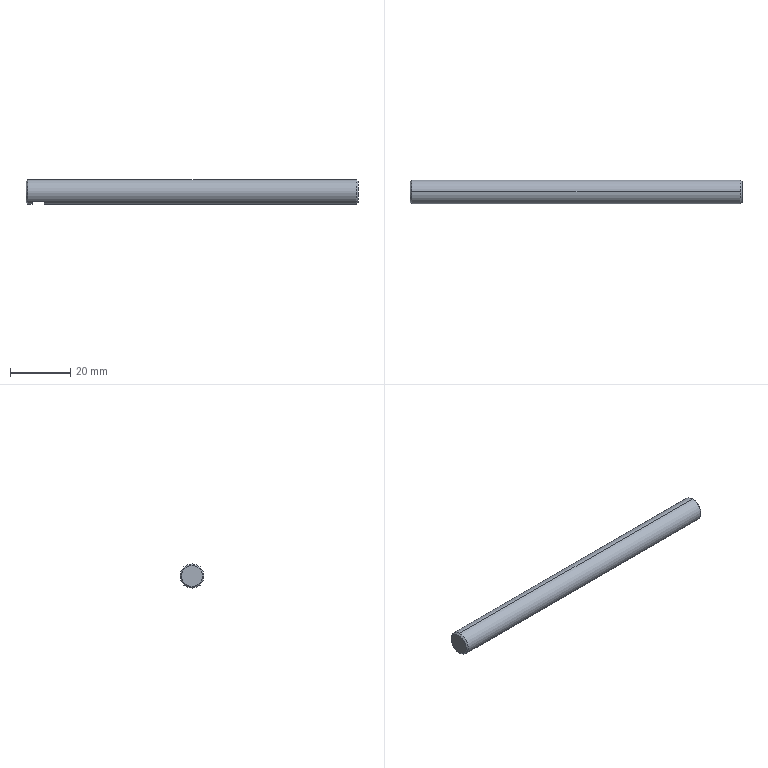Part | SolidWorks | features Chamfer 1, ICE 1, Revolution 1 | 1 solid | 11 faces | box 110 x 8 x 8 mm | volume 5509 mm3 | plane 5 | cone 4 | cylinder 2 | commonest cylinder face diameters 8 x2
STEP:
#1=CARTESIAN_POINT('',(0.,0.,3.5));
#2=VERTEX_POINT('',#1);
#3=CARTESIAN_POINT('',(0.,0.,-3.5));
#4=VERTEX_POINT('',#3);
#5=CARTESIAN_POINT('',(0.,0.,0.));
#6=DIRECTION('',(-1.,0.,0.));
#7=DIRECTION('',(0.,0.,-1.));
#8=AXIS2_PLACEMENT_3D('',#5,#6,#7);
#9=CIRCLE('',#8,3.5);
#10=EDGE_CURVE('',#2,#4,#9,.T.);
#11=ORIENTED_EDGE('',*,*,#10,.F.);
#12=CARTESIAN_POINT('',(0.5,0.,4.));
#13=VERTEX_POINT('',#12);
#14=CARTESIAN_POINT('',(0.,0.,3.5));
#15=DIRECTION('',(0.7071,0.,0.7071));
#16=VECTOR('',#15,1000.);
#17=LINE('',#14,#16);
#18=EDGE_CURVE('',#2,#13,#17,.T.);
#19=ORIENTED_EDGE('',*,*,#18,.T.);
#20=CARTESIAN_POINT('',(0.5,0.,-4.));
#21=VERTEX_POINT('',#20);
#22=CARTESIAN_POINT('',(0.5,0.,0.));
#23=DIRECTION('',(1.,0.,0.));
#24=DIRECTION('',(0.,0.,-1.));
#25=AXIS2_PLACEMENT_3D('',#22,#23,#24);
#26=CIRCLE('',#25,4.);
#27=EDGE_CURVE('',#21,#13,#26,.T.);
#28=ORIENTED_EDGE('',*,*,#27,.F.);
#29=CARTESIAN_POINT('',(0.,0.,-3.5));
#30=DIRECTION('',(0.7071,0.,-0.7071));
#31=VECTOR('',#30,1000.);
#32=LINE('',#29,#31);
#33=EDGE_CURVE('',#4,#21,#32,.T.);
#34=ORIENTED_EDGE('',*,*,#33,.F.);
#35=EDGE_LOOP('',(#11,#19,#28,#34));
#36=FACE_OUTER_BOUND('',#35,.T.);
#37=CARTESIAN_POINT('',(0.,0.,0.));
#38=DIRECTION('',(1.,0.,0.));
#39=DIRECTION('',(0.,0.,-1.));
#40=AXIS2_PLACEMENT_3D('',#37,#38,#39);
#41=CONICAL_SURFACE('',#40,3.5,0.7854);
#42=ADVANCED_FACE('',(#36),#41,.T.);
#43=CARTESIAN_POINT('',(110.,0.,-3.5));
#44=VERTEX_POINT('',#43);
#45=CARTESIAN_POINT('',(110.,0.,3.5));
#46=VERTEX_POINT('',#45);
#47=CARTESIAN_POINT('',(110.,0.,0.));
#48=DIRECTION('',(1.,0.,0.));
#49=DIRECTION('',(0.,0.,1.));
#50=AXIS2_PLACEMENT_3D('',#47,#48,#49);
#51=CIRCLE('',#50,3.5);
#52=EDGE_CURVE('',#44,#46,#51,.T.);
#53=ORIENTED_EDGE('',*,*,#52,.F.);
#54=CARTESIAN_POINT('',(109.5,0.,-4.));
#55=VERTEX_POINT('',#54);
#56=CARTESIAN_POINT('',(109.5,0.,-4.));
#57=DIRECTION('',(-0.7071,0.,-0.7071));
#58=VECTOR('',#57,1000.);
#59=LINE('',#56,#58);
#60=EDGE_CURVE('',#44,#55,#59,.T.);
#61=ORIENTED_EDGE('',*,*,#60,.T.);
#62=CARTESIAN_POINT('',(109.5,0.,4.));
#63=VERTEX_POINT('',#62);
#64=CARTESIAN_POINT('',(109.5,0.,0.));
#65=DIRECTION('',(-1.,0.,0.));
#66=DIRECTION('',(0.,0.,1.));
#67=AXIS2_PLACEMENT_3D('',#64,#65,#66);
#68=CIRCLE('',#67,4.);
#69=EDGE_CURVE('',#63,#55,#68,.T.);
#70=ORIENTED_EDGE('',*,*,#69,.F.);
#71=CARTESIAN_POINT('',(109.5,0.,4.));
#72=DIRECTION('',(-0.7071,0.,0.7071));
#73=VECTOR('',#72,1000.);
#74=LINE('',#71,#73);
#75=EDGE_CURVE('',#46,#63,#74,.T.);
#76=ORIENTED_EDGE('',*,*,#75,.F.);
#77=EDGE_LOOP('',(#53,#61,#70,#76));
#78=FACE_OUTER_BOUND('',#77,.T.);
#79=CARTESIAN_POINT('',(109.5,0.,0.));
#80=DIRECTION('',(-1.,0.,0.));
#81=DIRECTION('',(0.,0.,1.));
#82=AXIS2_PLACEMENT_3D('',#79,#80,#81);
#83=CONICAL_SURFACE('',#82,4.,0.7854);
#84=ADVANCED_FACE('',(#78),#83,.T.);
#85=ORIENTED_EDGE('',*,*,#69,.T.);
#86=CARTESIAN_POINT('',(6.,0.,-4.));
#87=VERTEX_POINT('',#86);
#88=CARTESIAN_POINT('',(0.,0.,-4.));
#89=DIRECTION('',(-1.,0.,0.));
#90=VECTOR('',#89,1000.);
#91=LINE('',#88,#90);
#92=EDGE_CURVE('',#55,#87,#91,.T.);
#93=ORIENTED_EDGE('',*,*,#92,.T.);
#94=CARTESIAN_POINT('',(6.,2.646,-3.));
#95=VERTEX_POINT('',#94);
#96=CARTESIAN_POINT('',(6.,0.,0.));
#97=DIRECTION('',(1.,0.,0.));
#98=DIRECTION('',(0.,0.,-1.));
#99=AXIS2_PLACEMENT_3D('',#96,#97,#98);
#100=CIRCLE('',#99,4.);
#101=EDGE_CURVE('',#87,#95,#100,.T.);
#102=ORIENTED_EDGE('',*,*,#101,.T.);
#103=CARTESIAN_POINT('',(2.,2.646,-3.));
#104=VERTEX_POINT('',#103);
#105=CARTESIAN_POINT('',(0.,2.646,-3.));
#106=DIRECTION('',(-1.,0.,0.));
#107=VECTOR('',#106,1000.);
#108=LINE('',#105,#107);
#109=EDGE_CURVE('',#95,#104,#108,.T.);
#110=ORIENTED_EDGE('',*,*,#109,.T.);
#111=CARTESIAN_POINT('',(2.,0.,-4.));
#112=VERTEX_POINT('',#111);
#113=CARTESIAN_POINT('',(2.,0.,0.));
#114=DIRECTION('',(-1.,0.,0.));
#115=DIRECTION('',(0.,0.,1.));
#116=AXIS2_PLACEMENT_3D('',#113,#114,#115);
#117=CIRCLE('',#116,4.);
#118=EDGE_CURVE('',#104,#112,#117,.T.);
#119=ORIENTED_EDGE('',*,*,#118,.T.);
#120=CARTESIAN_POINT('',(0.,0.,-4.));
#121=DIRECTION('',(-1.,0.,0.));
#122=VECTOR('',#121,1000.);
#123=LINE('',#120,#122);
#124=EDGE_CURVE('',#112,#21,#123,.T.);
#125=ORIENTED_EDGE('',*,*,#124,.T.);
#126=ORIENTED_EDGE('',*,*,#27,.T.);
#127=CARTESIAN_POINT('',(0.,0.,4.));
#128=DIRECTION('',(-1.,0.,0.));
#129=VECTOR('',#128,1000.);
#130=LINE('',#127,#129);
#131=EDGE_CURVE('',#63,#13,#130,.T.);
#132=ORIENTED_EDGE('',*,*,#131,.F.);
#133=EDGE_LOOP('',(#85,#93,#102,#110,#119,#125,#126,#132));
#134=FACE_OUTER_BOUND('',#133,.T.);
#135=CARTESIAN_POINT('',(0.,0.,0.));
#136=DIRECTION('',(-1.,0.,0.));
#137=DIRECTION('',(0.,0.,1.));
#138=AXIS2_PLACEMENT_3D('',#135,#136,#137);
#139=CYLINDRICAL_SURFACE('',#138,4.);
#140=ADVANCED_FACE('',(#134),#139,.T.);
#141=CARTESIAN_POINT('',(0.,0.,0.));
#142=DIRECTION('',(-1.,0.,0.));
#143=DIRECTION('',(0.,0.,-1.));
#144=AXIS2_PLACEMENT_3D('',#141,#142,#143);
#145=CIRCLE('',#144,3.5);
#146=EDGE_CURVE('',#4,#2,#145,.T.);
#147=ORIENTED_EDGE('',*,*,#146,.T.);
#148=ORIENTED_EDGE('',*,*,#10,.T.);
#149=EDGE_LOOP('',(#147,#148));
#150=FACE_OUTER_BOUND('',#149,.T.);
#151=CARTESIAN_POINT('',(0.,0.,0.));
#152=DIRECTION('',(1.,0.,0.));
#153=DIRECTION('',(0.,0.,-1.));
#154=AXIS2_PLACEMENT_3D('',#151,#152,#153);
#155=PLANE('',#154);
#156=ADVANCED_FACE('',(#150),#155,.F.);
#157=ORIENTED_EDGE('',*,*,#92,.F.);
#158=CARTESIAN_POINT('',(109.5,0.,0.));
#159=DIRECTION('',(-1.,0.,0.));
#160=DIRECTION('',(0.,0.,1.));
#161=AXIS2_PLACEMENT_3D('',#158,#159,#160);
#162=CIRCLE('',#161,4.);
#163=EDGE_CURVE('',#55,#63,#162,.T.);
#164=ORIENTED_EDGE('',*,*,#163,.T.);
#165=ORIENTED_EDGE('',*,*,#131,.T.);
#166=CARTESIAN_POINT('',(0.5,0.,0.));
#167=DIRECTION('',(1.,0.,0.));
#168=DIRECTION('',(0.,0.,-1.));
#169=AXIS2_PLACEMENT_3D('',#166,#167,#168);
#170=CIRCLE('',#169,4.);
#171=EDGE_CURVE('',#13,#21,#170,.T.);
#172=ORIENTED_EDGE('',*,*,#171,.T.);
#173=ORIENTED_EDGE('',*,*,#124,.F.);
#174=CARTESIAN_POINT('',(2.,-2.646,-3.));
#175=VERTEX_POINT('',#174);
#176=CARTESIAN_POINT('',(2.,0.,0.));
#177=DIRECTION('',(-1.,0.,0.));
#178=DIRECTION('',(0.,0.,1.));
#179=AXIS2_PLACEMENT_3D('',#176,#177,#178);
#180=CIRCLE('',#179,4.);
#181=EDGE_CURVE('',#112,#175,#180,.T.);
#182=ORIENTED_EDGE('',*,*,#181,.T.);
#183=CARTESIAN_POINT('',(6.,-2.646,-3.));
#184=VERTEX_POINT('',#183);
#185=CARTESIAN_POINT('',(0.,-2.646,-3.));
#186=DIRECTION('',(1.,0.,0.));
#187=VECTOR('',#186,1000.);
#188=LINE('',#185,#187);
#189=EDGE_CURVE('',#175,#184,#188,.T.);
#190=ORIENTED_EDGE('',*,*,#189,.T.);
#191=CARTESIAN_POINT('',(6.,0.,0.));
#192=DIRECTION('',(1.,0.,0.));
#193=DIRECTION('',(0.,0.,-1.));
#194=AXIS2_PLACEMENT_3D('',#191,#192,#193);
#195=CIRCLE('',#194,4.);
#196=EDGE_CURVE('',#184,#87,#195,.T.);
#197=ORIENTED_EDGE('',*,*,#196,.T.);
#198=EDGE_LOOP('',(#157,#164,#165,#172,#173,#182,#190,#197));
#199=FACE_OUTER_BOUND('',#198,.T.);
#200=CARTESIAN_POINT('',(0.,0.,0.));
#201=DIRECTION('',(-1.,0.,0.));
#202=DIRECTION('',(0.,0.,1.));
#203=AXIS2_PLACEMENT_3D('',#200,#201,#202);
#204=CYLINDRICAL_SURFACE('',#203,4.);
#205=ADVANCED_FACE('',(#199),#204,.T.);
#206=CARTESIAN_POINT('',(110.,0.,0.));
#207=DIRECTION('',(1.,0.,0.));
#208=DIRECTION('',(0.,0.,1.));
#209=AXIS2_PLACEMENT_3D('',#206,#207,#208);
#210=CIRCLE('',#209,3.5);
#211=EDGE_CURVE('',#46,#44,#210,.T.);
#212=ORIENTED_EDGE('',*,*,#211,.T.);
#213=ORIENTED_EDGE('',*,*,#52,.T.);
#214=EDGE_LOOP('',(#212,#213));
#215=FACE_OUTER_BOUND('',#214,.T.);
#216=CARTESIAN_POINT('',(110.,4.,0.));
#217=DIRECTION('',(-1.,0.,0.));
#218=DIRECTION('',(0.,0.,1.));
#219=AXIS2_PLACEMENT_3D('',#216,#217,#218);
#220=PLANE('',#219);
#221=ADVANCED_FACE('',(#215),#220,.F.);
#222=CARTESIAN_POINT('',(6.,-5.,-3.));
#223=DIRECTION('',(0.,1.,0.));
#224=VECTOR('',#223,1000.);
#225=LINE('',#222,#224);
#226=EDGE_CURVE('',#184,#95,#225,.T.);
#227=ORIENTED_EDGE('',*,*,#226,.T.);
#228=ORIENTED_EDGE('',*,*,#101,.F.);
#229=ORIENTED_EDGE('',*,*,#196,.F.);
#230=EDGE_LOOP('',(#227,#228,#229));
#231=FACE_OUTER_BOUND('',#230,.T.);
#232=CARTESIAN_POINT('',(6.,-5.,-3.));
#233=DIRECTION('',(1.,0.,0.));
#234=DIRECTION('',(0.,0.,-1.));
#235=AXIS2_PLACEMENT_3D('',#232,#233,#234);
#236=PLANE('',#235);
#237=ADVANCED_FACE('',(#231),#236,.F.);
#238=ORIENTED_EDGE('',*,*,#226,.F.);
#239=ORIENTED_EDGE('',*,*,#189,.F.);
#240=CARTESIAN_POINT('',(2.,-5.,-3.));
#241=DIRECTION('',(0.,1.,0.));
#242=VECTOR('',#241,1000.);
#243=LINE('',#240,#242);
#244=EDGE_CURVE('',#175,#104,#243,.T.);
#245=ORIENTED_EDGE('',*,*,#244,.T.);
#246=ORIENTED_EDGE('',*,*,#109,.F.);
#247=EDGE_LOOP('',(#238,#239,#245,#246));
#248=FACE_OUTER_BOUND('',#247,.T.);
#249=CARTESIAN_POINT('',(2.,-5.,-3.));
#250=DIRECTION('',(0.,0.,1.));
#251=DIRECTION('',(1.,0.,0.));
#252=AXIS2_PLACEMENT_3D('',#249,#250,#251);
#253=PLANE('',#252);
#254=ADVANCED_FACE('',(#248),#253,.F.);
#255=ORIENTED_EDGE('',*,*,#244,.F.);
#256=ORIENTED_EDGE('',*,*,#181,.F.);
#257=ORIENTED_EDGE('',*,*,#118,.F.);
#258=EDGE_LOOP('',(#255,#256,#257));
#259=FACE_OUTER_BOUND('',#258,.T.);
#260=CARTESIAN_POINT('',(2.,-5.,-3.));
#261=DIRECTION('',(-1.,0.,0.));
#262=DIRECTION('',(0.,0.,1.));
#263=AXIS2_PLACEMENT_3D('',#260,#261,#262);
#264=PLANE('',#263);
#265=ADVANCED_FACE('',(#259),#264,.F.);
#266=ORIENTED_EDGE('',*,*,#60,.F.);
#267=ORIENTED_EDGE('',*,*,#211,.F.);
#268=ORIENTED_EDGE('',*,*,#75,.T.);
#269=ORIENTED_EDGE('',*,*,#163,.F.);
#270=EDGE_LOOP('',(#266,#267,#268,#269));
#271=FACE_OUTER_BOUND('',#270,.T.);
#272=CARTESIAN_POINT('',(109.5,0.,0.));
#273=DIRECTION('',(-1.,0.,0.));
#274=DIRECTION('',(0.,0.,1.));
#275=AXIS2_PLACEMENT_3D('',#272,#273,#274);
#276=CONICAL_SURFACE('',#275,4.,0.7854);
#277=ADVANCED_FACE('',(#271),#276,.T.);
#278=ORIENTED_EDGE('',*,*,#18,.F.);
#279=ORIENTED_EDGE('',*,*,#146,.F.);
#280=ORIENTED_EDGE('',*,*,#33,.T.);
#281=ORIENTED_EDGE('',*,*,#171,.F.);
#282=EDGE_LOOP('',(#278,#279,#280,#281));
#283=FACE_OUTER_BOUND('',#282,.T.);
#284=CARTESIAN_POINT('',(0.,0.,0.));
#285=DIRECTION('',(1.,0.,0.));
#286=DIRECTION('',(0.,0.,-1.));
#287=AXIS2_PLACEMENT_3D('',#284,#285,#286);
#288=CONICAL_SURFACE('',#287,3.5,0.7854);
#289=ADVANCED_FACE('',(#283),#288,.T.);
#290=CLOSED_SHELL('',(#42,#84,#140,#156,#205,#221,#237,#254,#265,#277,#289));
#291=MANIFOLD_SOLID_BREP('',#290);
#292=CARTESIAN_POINT('',(0.,0.,0.));
#293=DIRECTION('',(0.,0.,1.));
#294=DIRECTION('',(1.,0.,0.));
#295=AXIS2_PLACEMENT_3D('',#292,#293,#294);
#296=(LENGTH_UNIT()NAMED_UNIT(*)SI_UNIT(.MILLI.,.METRE.));
#297=UNCERTAINTY_MEASURE_WITH_UNIT(LENGTH_MEASURE(0.00001),#296,'','');
#298=(NAMED_UNIT(*)PLANE_ANGLE_UNIT()SI_UNIT($,.RADIAN.));
#299=(NAMED_UNIT(*)SI_UNIT($,.STERADIAN.)SOLID_ANGLE_UNIT());
#300=(GEOMETRIC_REPRESENTATION_CONTEXT(3)GLOBAL_UNCERTAINTY_ASSIGNED_CONTEXT((#297))GLOBAL_UNIT_ASSIGNED_CONTEXT((#296,#298,#299))REPRESENTATION_CONTEXT('',''));
#301=ADVANCED_BREP_SHAPE_REPRESENTATION('',(#291,#295),#300);